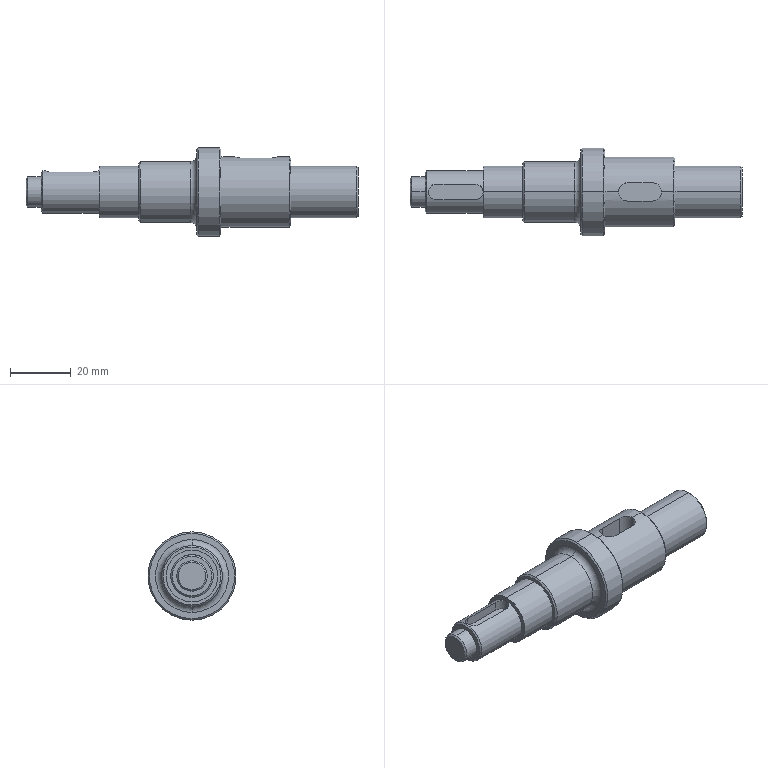Part | SolidWorks | features ICE 8, Chamfer 1, Extrusion 1, Fillet 1 | 1 solid | 50 faces | box 109 x 29 x 29 mm | volume 31302 mm3 | cylinder 20 | cone 14 | plane 14 | torus 2 | commonest cylinder face diameters 17 x4 5 x3 6 x3 10 x2 14 x2 20 x2
STEP:
#1=CARTESIAN_POINT('',(56.,0.,12.));
#2=VERTEX_POINT('',#1);
#3=CARTESIAN_POINT('',(56.,0.,-12.));
#4=VERTEX_POINT('',#3);
#5=CARTESIAN_POINT('',(56.,0.,0.));
#6=DIRECTION('',(1.,0.,0.));
#7=DIRECTION('',(0.,0.,-1.));
#8=AXIS2_PLACEMENT_3D('',#5,#6,#7);
#9=CIRCLE('',#8,12.);
#10=EDGE_CURVE('',#2,#4,#9,.T.);
#11=ORIENTED_EDGE('',*,*,#10,.F.);
#12=CARTESIAN_POINT('',(54.,0.,10.));
#13=VERTEX_POINT('',#12);
#14=CARTESIAN_POINT('',(54.,0.,12.));
#15=DIRECTION('',(0.,1.,0.));
#16=DIRECTION('',(0.,0.,1.));
#17=AXIS2_PLACEMENT_3D('',#14,#15,#16);
#18=CIRCLE('',#17,2.);
#19=EDGE_CURVE('',#2,#13,#18,.T.);
#20=ORIENTED_EDGE('',*,*,#19,.T.);
#21=CARTESIAN_POINT('',(54.,0.,-10.));
#22=VERTEX_POINT('',#21);
#23=CARTESIAN_POINT('',(54.,0.,0.));
#24=DIRECTION('',(-1.,0.,0.));
#25=DIRECTION('',(0.,0.,-1.));
#26=AXIS2_PLACEMENT_3D('',#23,#24,#25);
#27=CIRCLE('',#26,10.);
#28=EDGE_CURVE('',#22,#13,#27,.T.);
#29=ORIENTED_EDGE('',*,*,#28,.F.);
#30=CARTESIAN_POINT('',(54.,0.,-12.));
#31=DIRECTION('',(0.,-1.,0.));
#32=DIRECTION('',(0.,0.,-1.));
#33=AXIS2_PLACEMENT_3D('',#30,#31,#32);
#34=CIRCLE('',#33,2.);
#35=EDGE_CURVE('',#4,#22,#34,.T.);
#36=ORIENTED_EDGE('',*,*,#35,.F.);
#37=EDGE_LOOP('',(#11,#20,#29,#36));
#38=FACE_OUTER_BOUND('',#37,.T.);
#39=CARTESIAN_POINT('',(54.,0.,0.));
#40=DIRECTION('',(1.,0.,0.));
#41=DIRECTION('',(0.,0.,-1.));
#42=AXIS2_PLACEMENT_3D('',#39,#40,#41);
#43=TOROIDAL_SURFACE('',#42,12.,2.);
#44=ADVANCED_FACE('',(#38),#43,.F.);
#45=CARTESIAN_POINT('',(82.5,0.,5.));
#46=VERTEX_POINT('',#45);
#47=CARTESIAN_POINT('',(79.5,3.,5.));
#48=VERTEX_POINT('',#47);
#49=CARTESIAN_POINT('',(79.5,0.,5.));
#50=DIRECTION('',(0.,0.,1.));
#51=DIRECTION('',(1.,0.,0.));
#52=AXIS2_PLACEMENT_3D('',#49,#50,#51);
#53=CIRCLE('',#52,3.);
#54=EDGE_CURVE('',#46,#48,#53,.T.);
#55=ORIENTED_EDGE('',*,*,#54,.F.);
#56=CARTESIAN_POINT('',(82.5,0.,11.5));
#57=VERTEX_POINT('',#56);
#58=CARTESIAN_POINT('',(82.5,0.,5.));
#59=DIRECTION('',(0.,0.,1.));
#60=VECTOR('',#59,1000.);
#61=LINE('',#58,#60);
#62=EDGE_CURVE('',#46,#57,#61,.T.);
#63=ORIENTED_EDGE('',*,*,#62,.T.);
#64=CARTESIAN_POINT('',(79.5,3.,11.102));
#65=VERTEX_POINT('',#64);
#66=CARTESIAN_POINT('',(79.5,3.,11.102));
#67=CARTESIAN_POINT('',(79.699,3.,11.102));
#68=CARTESIAN_POINT('',(79.895,2.98,11.107));
#69=CARTESIAN_POINT('',(80.28,2.904,11.127));
#70=CARTESIAN_POINT('',(80.471,2.845,11.143));
#71=CARTESIAN_POINT('',(80.834,2.694,11.18));
#72=CARTESIAN_POINT('',(81.006,2.602,11.202));
#73=CARTESIAN_POINT('',(81.331,2.384,11.251));
#74=CARTESIAN_POINT('',(81.485,2.258,11.277));
#75=CARTESIAN_POINT('',(81.76,1.983,11.329));
#76=CARTESIAN_POINT('',(81.884,1.832,11.354));
#77=CARTESIAN_POINT('',(82.103,1.504,11.402));
#78=CARTESIAN_POINT('',(82.196,1.331,11.424));
#79=CARTESIAN_POINT('',(82.346,0.97,11.46));
#80=CARTESIAN_POINT('',(82.404,0.7798,11.475));
#81=CARTESIAN_POINT('',(82.481,0.392,11.495));
#82=CARTESIAN_POINT('',(82.5,0.1967,11.5));
#83=CARTESIAN_POINT('',(82.5,0.,11.5));
#84=B_SPLINE_CURVE_WITH_KNOTS('',3,(#66,#67,#68,#69,#70,#71,#72,#73,#74,#75,#76,#77,#78,#79,#80,#81,#82,#83),.UNSPECIFIED.,.F.,.F.,(4,2,2,2,2,2,2,2,4),(0.,0.0005889,0.001178,0.001767,0.002356,0.002945,0.003533,0.004122,0.004711),.UNSPECIFIED.);
#85=EDGE_CURVE('',#65,#57,#84,.T.);
#86=ORIENTED_EDGE('',*,*,#85,.F.);
#87=CARTESIAN_POINT('',(79.5,3.,5.));
#88=DIRECTION('',(0.,0.,1.));
#89=VECTOR('',#88,1000.);
#90=LINE('',#87,#89);
#91=EDGE_CURVE('',#48,#65,#90,.T.);
#92=ORIENTED_EDGE('',*,*,#91,.F.);
#93=EDGE_LOOP('',(#55,#63,#86,#92));
#94=FACE_OUTER_BOUND('',#93,.T.);
#95=CARTESIAN_POINT('',(79.5,0.,5.));
#96=DIRECTION('',(0.,0.,1.));
#97=DIRECTION('',(1.,0.,0.));
#98=AXIS2_PLACEMENT_3D('',#95,#96,#97);
#99=CYLINDRICAL_SURFACE('',#98,3.);
#100=ADVANCED_FACE('',(#94),#99,.F.);
#101=CARTESIAN_POINT('',(24.,0.,3.5));
#102=VERTEX_POINT('',#101);
#103=CARTESIAN_POINT('',(21.5,2.5,3.5));
#104=VERTEX_POINT('',#103);
#105=CARTESIAN_POINT('',(21.5,0.,3.5));
#106=DIRECTION('',(0.,0.,1.));
#107=DIRECTION('',(1.,0.,0.));
#108=AXIS2_PLACEMENT_3D('',#105,#106,#107);
#109=CIRCLE('',#108,2.5);
#110=EDGE_CURVE('',#102,#104,#109,.T.);
#111=ORIENTED_EDGE('',*,*,#110,.F.);
#112=CARTESIAN_POINT('',(24.,0.,7.));
#113=VERTEX_POINT('',#112);
#114=CARTESIAN_POINT('',(24.,0.,3.5));
#115=DIRECTION('',(0.,0.,1.));
#116=VECTOR('',#115,1000.);
#117=LINE('',#114,#116);
#118=EDGE_CURVE('',#102,#113,#117,.T.);
#119=ORIENTED_EDGE('',*,*,#118,.T.);
#120=CARTESIAN_POINT('',(21.5,2.5,6.538));
#121=VERTEX_POINT('',#120);
#122=CARTESIAN_POINT('',(21.5,2.5,6.538));
#123=CARTESIAN_POINT('',(21.667,2.5,6.538));
#124=CARTESIAN_POINT('',(21.83,2.484,6.545));
#125=CARTESIAN_POINT('',(22.151,2.419,6.569));
#126=CARTESIAN_POINT('',(22.311,2.371,6.587));
#127=CARTESIAN_POINT('',(22.612,2.245,6.631));
#128=CARTESIAN_POINT('',(22.755,2.168,6.656));
#129=CARTESIAN_POINT('',(23.026,1.987,6.713));
#130=CARTESIAN_POINT('',(23.153,1.883,6.743));
#131=CARTESIAN_POINT('',(23.496,1.54,6.833));
#132=CARTESIAN_POINT('',(23.681,1.264,6.892));
#133=CARTESIAN_POINT('',(23.87,0.8135,6.954));
#134=CARTESIAN_POINT('',(23.918,0.6548,6.971));
#135=CARTESIAN_POINT('',(23.984,0.3308,6.994));
#136=CARTESIAN_POINT('',(24.,0.1666,7.));
#137=CARTESIAN_POINT('',(24.,0.,7.));
#138=B_SPLINE_CURVE_WITH_KNOTS('',3,(#122,#123,#124,#125,#126,#127,#128,#129,#130,#131,#132,#133,#134,#135,#136,#137),.UNSPECIFIED.,.F.,.F.,(4,2,2,2,2,2,2,4),(0.,0.0004923,0.0009846,0.001477,0.001969,0.002954,0.003446,0.003938),.UNSPECIFIED.);
#139=EDGE_CURVE('',#121,#113,#138,.T.);
#140=ORIENTED_EDGE('',*,*,#139,.F.);
#141=CARTESIAN_POINT('',(21.5,2.5,3.5));
#142=DIRECTION('',(0.,0.,1.));
#143=VECTOR('',#142,1000.);
#144=LINE('',#141,#143);
#145=EDGE_CURVE('',#104,#121,#144,.T.);
#146=ORIENTED_EDGE('',*,*,#145,.F.);
#147=EDGE_LOOP('',(#111,#119,#140,#146));
#148=FACE_OUTER_BOUND('',#147,.T.);
#149=CARTESIAN_POINT('',(21.5,0.,3.5));
#150=DIRECTION('',(0.,0.,1.));
#151=DIRECTION('',(1.,0.,0.));
#152=AXIS2_PLACEMENT_3D('',#149,#150,#151);
#153=CYLINDRICAL_SURFACE('',#152,2.5);
#154=ADVANCED_FACE('',(#148),#153,.F.);
#155=CARTESIAN_POINT('',(5.,0.,6.5));
#156=VERTEX_POINT('',#155);
#157=CARTESIAN_POINT('',(5.,0.,-6.5));
#158=VERTEX_POINT('',#157);
#159=CARTESIAN_POINT('',(5.,0.,0.));
#160=DIRECTION('',(-1.,0.,0.));
#161=DIRECTION('',(0.,0.,-1.));
#162=AXIS2_PLACEMENT_3D('',#159,#160,#161);
#163=CIRCLE('',#162,6.5);
#164=EDGE_CURVE('',#156,#158,#163,.T.);
#165=ORIENTED_EDGE('',*,*,#164,.F.);
#166=CARTESIAN_POINT('',(5.5,0.,7.));
#167=VERTEX_POINT('',#166);
#168=CARTESIAN_POINT('',(5.5,0.,7.));
#169=DIRECTION('',(0.7071,0.,0.7071));
#170=VECTOR('',#169,1000.);
#171=LINE('',#168,#170);
#172=EDGE_CURVE('',#156,#167,#171,.T.);
#173=ORIENTED_EDGE('',*,*,#172,.T.);
#174=CARTESIAN_POINT('',(5.5,0.,-7.));
#175=VERTEX_POINT('',#174);
#176=CARTESIAN_POINT('',(5.5,0.,0.));
#177=DIRECTION('',(1.,0.,0.));
#178=DIRECTION('',(0.,0.,-1.));
#179=AXIS2_PLACEMENT_3D('',#176,#177,#178);
#180=CIRCLE('',#179,7.);
#181=EDGE_CURVE('',#175,#167,#180,.T.);
#182=ORIENTED_EDGE('',*,*,#181,.F.);
#183=CARTESIAN_POINT('',(5.5,0.,-7.));
#184=DIRECTION('',(0.7071,0.,-0.7071));
#185=VECTOR('',#184,1000.);
#186=LINE('',#183,#185);
#187=EDGE_CURVE('',#158,#175,#186,.T.);
#188=ORIENTED_EDGE('',*,*,#187,.F.);
#189=EDGE_LOOP('',(#165,#173,#182,#188));
#190=FACE_OUTER_BOUND('',#189,.T.);
#191=CARTESIAN_POINT('',(5.5,0.,0.));
#192=DIRECTION('',(1.,0.,0.));
#193=DIRECTION('',(0.,0.,-1.));
#194=AXIS2_PLACEMENT_3D('',#191,#192,#193);
#195=CONICAL_SURFACE('',#194,7.,0.7854);
#196=ADVANCED_FACE('',(#190),#195,.T.);
#197=CARTESIAN_POINT('',(37.,0.,9.5));
#198=VERTEX_POINT('',#197);
#199=CARTESIAN_POINT('',(37.,0.,-9.5));
#200=VERTEX_POINT('',#199);
#201=CARTESIAN_POINT('',(37.,0.,0.));
#202=DIRECTION('',(-1.,0.,0.));
#203=DIRECTION('',(0.,0.,-1.));
#204=AXIS2_PLACEMENT_3D('',#201,#202,#203);
#205=CIRCLE('',#204,9.5);
#206=EDGE_CURVE('',#198,#200,#205,.T.);
#207=ORIENTED_EDGE('',*,*,#206,.F.);
#208=CARTESIAN_POINT('',(37.5,0.,10.));
#209=VERTEX_POINT('',#208);
#210=CARTESIAN_POINT('',(37.5,0.,10.));
#211=DIRECTION('',(0.7071,0.,0.7071));
#212=VECTOR('',#211,1000.);
#213=LINE('',#210,#212);
#214=EDGE_CURVE('',#198,#209,#213,.T.);
#215=ORIENTED_EDGE('',*,*,#214,.T.);
#216=CARTESIAN_POINT('',(37.5,0.,-10.));
#217=VERTEX_POINT('',#216);
#218=CARTESIAN_POINT('',(37.5,0.,0.));
#219=DIRECTION('',(1.,0.,0.));
#220=DIRECTION('',(0.,0.,-1.));
#221=AXIS2_PLACEMENT_3D('',#218,#219,#220);
#222=CIRCLE('',#221,10.);
#223=EDGE_CURVE('',#217,#209,#222,.T.);
#224=ORIENTED_EDGE('',*,*,#223,.F.);
#225=CARTESIAN_POINT('',(37.5,0.,-10.));
#226=DIRECTION('',(0.7071,0.,-0.7071));
#227=VECTOR('',#226,1000.);
#228=LINE('',#225,#227);
#229=EDGE_CURVE('',#200,#217,#228,.T.);
#230=ORIENTED_EDGE('',*,*,#229,.F.);
#231=EDGE_LOOP('',(#207,#215,#224,#230));
#232=FACE_OUTER_BOUND('',#231,.T.);
#233=CARTESIAN_POINT('',(37.5,0.,0.));
#234=DIRECTION('',(1.,0.,0.));
#235=DIRECTION('',(0.,0.,-1.));
#236=AXIS2_PLACEMENT_3D('',#233,#234,#235);
#237=CONICAL_SURFACE('',#236,10.,0.7854);
#238=ADVANCED_FACE('',(#232),#237,.T.);
#239=CARTESIAN_POINT('',(56.,0.,14.));
#240=VERTEX_POINT('',#239);
#241=CARTESIAN_POINT('',(56.,0.,-14.));
#242=VERTEX_POINT('',#241);
#243=CARTESIAN_POINT('',(56.,0.,0.));
#244=DIRECTION('',(-1.,0.,0.));
#245=DIRECTION('',(0.,0.,-1.));
#246=AXIS2_PLACEMENT_3D('',#243,#244,#245);
#247=CIRCLE('',#246,14.);
#248=EDGE_CURVE('',#240,#242,#247,.T.);
#249=ORIENTED_EDGE('',*,*,#248,.F.);
#250=CARTESIAN_POINT('',(56.5,0.,14.5));
#251=VERTEX_POINT('',#250);
#252=CARTESIAN_POINT('',(56.5,0.,14.5));
#253=DIRECTION('',(0.7071,0.,0.7071));
#254=VECTOR('',#253,1000.);
#255=LINE('',#252,#254);
#256=EDGE_CURVE('',#240,#251,#255,.T.);
#257=ORIENTED_EDGE('',*,*,#256,.T.);
#258=CARTESIAN_POINT('',(56.5,0.,-14.5));
#259=VERTEX_POINT('',#258);
#260=CARTESIAN_POINT('',(56.5,0.,0.));
#261=DIRECTION('',(1.,0.,0.));
#262=DIRECTION('',(0.,0.,-1.));
#263=AXIS2_PLACEMENT_3D('',#260,#261,#262);
#264=CIRCLE('',#263,14.5);
#265=EDGE_CURVE('',#259,#251,#264,.T.);
#266=ORIENTED_EDGE('',*,*,#265,.F.);
#267=CARTESIAN_POINT('',(56.5,0.,-14.5));
#268=DIRECTION('',(0.7071,0.,-0.7071));
#269=VECTOR('',#268,1000.);
#270=LINE('',#267,#269);
#271=EDGE_CURVE('',#242,#259,#270,.T.);
#272=ORIENTED_EDGE('',*,*,#271,.F.);
#273=EDGE_LOOP('',(#249,#257,#266,#272));
#274=FACE_OUTER_BOUND('',#273,.T.);
#275=CARTESIAN_POINT('',(56.5,0.,0.));
#276=DIRECTION('',(1.,0.,0.));
#277=DIRECTION('',(0.,0.,-1.));
#278=AXIS2_PLACEMENT_3D('',#275,#276,#277);
#279=CONICAL_SURFACE('',#278,14.5,0.7854);
#280=ADVANCED_FACE('',(#274),#279,.T.);
#281=CARTESIAN_POINT('',(64.,0.,-14.));
#282=VERTEX_POINT('',#281);
#283=CARTESIAN_POINT('',(64.,0.,14.));
#284=VERTEX_POINT('',#283);
#285=CARTESIAN_POINT('',(64.,0.,0.));
#286=DIRECTION('',(1.,0.,0.));
#287=DIRECTION('',(0.,0.,-1.));
#288=AXIS2_PLACEMENT_3D('',#285,#286,#287);
#289=CIRCLE('',#288,14.);
#290=EDGE_CURVE('',#282,#284,#289,.T.);
#291=ORIENTED_EDGE('',*,*,#290,.F.);
#292=CARTESIAN_POINT('',(63.5,0.,-14.5));
#293=VERTEX_POINT('',#292);
#294=CARTESIAN_POINT('',(64.,0.,-14.));
#295=DIRECTION('',(-0.7071,0.,-0.7071));
#296=VECTOR('',#295,1000.);
#297=LINE('',#294,#296);
#298=EDGE_CURVE('',#282,#293,#297,.T.);
#299=ORIENTED_EDGE('',*,*,#298,.T.);
#300=CARTESIAN_POINT('',(63.5,0.,14.5));
#301=VERTEX_POINT('',#300);
#302=CARTESIAN_POINT('',(63.5,0.,0.));
#303=DIRECTION('',(-1.,0.,0.));
#304=DIRECTION('',(0.,0.,-1.));
#305=AXIS2_PLACEMENT_3D('',#302,#303,#304);
#306=CIRCLE('',#305,14.5);
#307=EDGE_CURVE('',#301,#293,#306,.T.);
#308=ORIENTED_EDGE('',*,*,#307,.F.);
#309=CARTESIAN_POINT('',(64.,0.,14.));
#310=DIRECTION('',(-0.7071,0.,0.7071));
#311=VECTOR('',#310,1000.);
#312=LINE('',#309,#311);
#313=EDGE_CURVE('',#284,#301,#312,.T.);
#314=ORIENTED_EDGE('',*,*,#313,.F.);
#315=EDGE_LOOP('',(#291,#299,#308,#314));
#316=FACE_OUTER_BOUND('',#315,.T.);
#317=CARTESIAN_POINT('',(64.,0.,0.));
#318=DIRECTION('',(-1.,0.,0.));
#319=DIRECTION('',(0.,0.,1.));
#320=AXIS2_PLACEMENT_3D('',#317,#318,#319);
#321=CONICAL_SURFACE('',#320,14.,0.7854);
#322=ADVANCED_FACE('',(#316),#321,.T.);
#323=CARTESIAN_POINT('',(87.,0.,-11.));
#324=VERTEX_POINT('',#323);
#325=CARTESIAN_POINT('',(87.,0.,11.));
#326=VERTEX_POINT('',#325);
#327=CARTESIAN_POINT('',(87.,0.,0.));
#328=DIRECTION('',(1.,0.,0.));
#329=DIRECTION('',(0.,0.,-1.));
#330=AXIS2_PLACEMENT_3D('',#327,#328,#329);
#331=CIRCLE('',#330,11.);
#332=EDGE_CURVE('',#324,#326,#331,.T.);
#333=ORIENTED_EDGE('',*,*,#332,.F.);
#334=CARTESIAN_POINT('',(86.5,0.,-11.5));
#335=VERTEX_POINT('',#334);
#336=CARTESIAN_POINT('',(87.,0.,-11.));
#337=DIRECTION('',(-0.7071,0.,-0.7071));
#338=VECTOR('',#337,1000.);
#339=LINE('',#336,#338);
#340=EDGE_CURVE('',#324,#335,#339,.T.);
#341=ORIENTED_EDGE('',*,*,#340,.T.);
#342=CARTESIAN_POINT('',(86.5,0.,11.5));
#343=VERTEX_POINT('',#342);
#344=CARTESIAN_POINT('',(86.5,0.,0.));
#345=DIRECTION('',(-1.,0.,0.));
#346=DIRECTION('',(0.,0.,-1.));
#347=AXIS2_PLACEMENT_3D('',#344,#345,#346);
#348=CIRCLE('',#347,11.5);
#349=EDGE_CURVE('',#343,#335,#348,.T.);
#350=ORIENTED_EDGE('',*,*,#349,.F.);
#351=CARTESIAN_POINT('',(87.,0.,11.));
#352=DIRECTION('',(-0.7071,0.,0.7071));
#353=VECTOR('',#352,1000.);
#354=LINE('',#351,#353);
#355=EDGE_CURVE('',#326,#343,#354,.T.);
#356=ORIENTED_EDGE('',*,*,#355,.F.);
#357=EDGE_LOOP('',(#333,#341,#350,#356));
#358=FACE_OUTER_BOUND('',#357,.T.);
#359=CARTESIAN_POINT('',(87.,0.,0.));
#360=DIRECTION('',(-1.,0.,0.));
#361=DIRECTION('',(0.,0.,1.));
#362=AXIS2_PLACEMENT_3D('',#359,#360,#361);
#363=CONICAL_SURFACE('',#362,11.,0.7854);
#364=ADVANCED_FACE('',(#358),#363,.T.);
#365=CARTESIAN_POINT('',(109.,0.,-8.));
#366=VERTEX_POINT('',#365);
#367=CARTESIAN_POINT('',(109.,0.,8.));
#368=VERTEX_POINT('',#367);
#369=CARTESIAN_POINT('',(109.,0.,0.));
#370=DIRECTION('',(1.,0.,0.));
#371=DIRECTION('',(0.,0.,-1.));
#372=AXIS2_PLACEMENT_3D('',#369,#370,#371);
#373=CIRCLE('',#372,8.);
#374=EDGE_CURVE('',#366,#368,#373,.T.);
#375=ORIENTED_EDGE('',*,*,#374,.F.);
#376=CARTESIAN_POINT('',(108.5,0.,-8.5));
#377=VERTEX_POINT('',#376);
#378=CARTESIAN_POINT('',(109.,0.,-8.));
#379=DIRECTION('',(-0.7071,0.,-0.7071));
#380=VECTOR('',#379,1000.);
#381=LINE('',#378,#380);
#382=EDGE_CURVE('',#366,#377,#381,.T.);
#383=ORIENTED_EDGE('',*,*,#382,.T.);
#384=CARTESIAN_POINT('',(108.5,0.,8.5));
#385=VERTEX_POINT('',#384);
#386=CARTESIAN_POINT('',(108.5,0.,0.));
#387=DIRECTION('',(-1.,0.,0.));
#388=DIRECTION('',(0.,0.,-1.));
#389=AXIS2_PLACEMENT_3D('',#386,#387,#388);
#390=CIRCLE('',#389,8.5);
#391=EDGE_CURVE('',#385,#377,#390,.T.);
#392=ORIENTED_EDGE('',*,*,#391,.F.);
#393=CARTESIAN_POINT('',(109.,0.,8.));
#394=DIRECTION('',(-0.7071,0.,0.7071));
#395=VECTOR('',#394,1000.);
#396=LINE('',#393,#395);
#397=EDGE_CURVE('',#368,#385,#396,.T.);
#398=ORIENTED_EDGE('',*,*,#397,.F.);
#399=EDGE_LOOP('',(#375,#383,#392,#398));
#400=FACE_OUTER_BOUND('',#399,.T.);
#401=CARTESIAN_POINT('',(109.,0.,0.));
#402=DIRECTION('',(-1.,0.,0.));
#403=DIRECTION('',(0.,0.,1.));
#404=AXIS2_PLACEMENT_3D('',#401,#402,#403);
#405=CONICAL_SURFACE('',#404,8.,0.7854);
#406=ADVANCED_FACE('',(#400),#405,.T.);
#407=CARTESIAN_POINT('',(0.,0.,4.5));
#408=VERTEX_POINT('',#407);
#409=CARTESIAN_POINT('',(0.,0.,-4.5));
#410=VERTEX_POINT('',#409);
#411=CARTESIAN_POINT('',(0.,0.,0.));
#412=DIRECTION('',(-1.,0.,0.));
#413=DIRECTION('',(0.,0.,-1.));
#414=AXIS2_PLACEMENT_3D('',#411,#412,#413);
#415=CIRCLE('',#414,4.5);
#416=EDGE_CURVE('',#408,#410,#415,.T.);
#417=ORIENTED_EDGE('',*,*,#416,.F.);
#418=CARTESIAN_POINT('',(0.5,0.,5.));
#419=VERTEX_POINT('',#418);
#420=CARTESIAN_POINT('',(0.5,0.,5.));
#421=DIRECTION('',(0.7071,0.,0.7071));
#422=VECTOR('',#421,1000.);
#423=LINE('',#420,#422);
#424=EDGE_CURVE('',#408,#419,#423,.T.);
#425=ORIENTED_EDGE('',*,*,#424,.T.);
#426=CARTESIAN_POINT('',(0.5,0.,-5.));
#427=VERTEX_POINT('',#426);
#428=CARTESIAN_POINT('',(0.5,0.,0.));
#429=DIRECTION('',(1.,0.,0.));
#430=DIRECTION('',(0.,0.,-1.));
#431=AXIS2_PLACEMENT_3D('',#428,#429,#430);
#432=CIRCLE('',#431,5.);
#433=EDGE_CURVE('',#427,#419,#432,.T.);
#434=ORIENTED_EDGE('',*,*,#433,.F.);
#435=CARTESIAN_POINT('',(0.5,0.,-5.));
#436=DIRECTION('',(0.7071,0.,-0.7071));
#437=VECTOR('',#436,1000.);
#438=LINE('',#435,#437);
#439=EDGE_CURVE('',#410,#427,#438,.T.);
#440=ORIENTED_EDGE('',*,*,#439,.F.);
#441=EDGE_LOOP('',(#417,#425,#434,#440));
#442=FACE_OUTER_BOUND('',#441,.T.);
#443=CARTESIAN_POINT('',(0.5,0.,0.));
#444=DIRECTION('',(1.,0.,0.));
#445=DIRECTION('',(0.,0.,-1.));
#446=AXIS2_PLACEMENT_3D('',#443,#444,#445);
#447=CONICAL_SURFACE('',#446,5.,0.7854);
#448=ADVANCED_FACE('',(#442),#447,.T.);
#449=ORIENTED_EDGE('',*,*,#391,.T.);
#450=CARTESIAN_POINT('',(87.,0.,-8.5));
#451=VERTEX_POINT('',#450);
#452=CARTESIAN_POINT('',(109.,0.,-8.5));
#453=DIRECTION('',(-1.,0.,0.));
#454=VECTOR('',#453,1000.);
#455=LINE('',#452,#454);
#456=EDGE_CURVE('',#377,#451,#455,.T.);
#457=ORIENTED_EDGE('',*,*,#456,.T.);
#458=CARTESIAN_POINT('',(87.,0.,8.5));
#459=VERTEX_POINT('',#458);
#460=CARTESIAN_POINT('',(87.,0.,0.));
#461=DIRECTION('',(1.,0.,0.));
#462=DIRECTION('',(0.,0.,-1.));
#463=AXIS2_PLACEMENT_3D('',#460,#461,#462);
#464=CIRCLE('',#463,8.5);
#465=EDGE_CURVE('',#451,#459,#464,.T.);
#466=ORIENTED_EDGE('',*,*,#465,.T.);
#467=CARTESIAN_POINT('',(109.,0.,8.5));
#468=DIRECTION('',(-1.,0.,0.));
#469=VECTOR('',#468,1000.);
#470=LINE('',#467,#469);
#471=EDGE_CURVE('',#385,#459,#470,.T.);
#472=ORIENTED_EDGE('',*,*,#471,.F.);
#473=EDGE_LOOP('',(#449,#457,#466,#472));
#474=FACE_OUTER_BOUND('',#473,.T.);
#475=CARTESIAN_POINT('',(109.,0.,0.));
#476=DIRECTION('',(-1.,0.,0.));
#477=DIRECTION('',(0.,0.,1.));
#478=AXIS2_PLACEMENT_3D('',#475,#476,#477);
#479=CYLINDRICAL_SURFACE('',#478,8.5);
#480=ADVANCED_FACE('',(#474),#479,.T.);
#481=ORIENTED_EDGE('',*,*,#349,.T.);
#482=CARTESIAN_POINT('',(64.,0.,-11.5));
#483=VERTEX_POINT('',#482);
#484=CARTESIAN_POINT('',(87.,0.,-11.5));
#485=DIRECTION('',(-1.,0.,0.));
#486=VECTOR('',#485,1000.);
#487=LINE('',#484,#486);
#488=EDGE_CURVE('',#335,#483,#487,.T.);
#489=ORIENTED_EDGE('',*,*,#488,.T.);
#490=CARTESIAN_POINT('',(64.,0.,11.5));
#491=VERTEX_POINT('',#490);
#492=CARTESIAN_POINT('',(64.,0.,0.));
#493=DIRECTION('',(1.,0.,0.));
#494=DIRECTION('',(0.,0.,-1.));
#495=AXIS2_PLACEMENT_3D('',#492,#493,#494);
#496=CIRCLE('',#495,11.5);
#497=EDGE_CURVE('',#483,#491,#496,.T.);
#498=ORIENTED_EDGE('',*,*,#497,.T.);
#499=CARTESIAN_POINT('',(68.5,0.,11.5));
#500=VERTEX_POINT('',#499);
#501=CARTESIAN_POINT('',(87.,0.,11.5));
#502=DIRECTION('',(-1.,0.,0.));
#503=VECTOR('',#502,1000.);
#504=LINE('',#501,#503);
#505=EDGE_CURVE('',#500,#491,#504,.T.);
#506=ORIENTED_EDGE('',*,*,#505,.F.);
#507=CARTESIAN_POINT('',(71.5,3.,11.102));
#508=VERTEX_POINT('',#507);
#509=CARTESIAN_POINT('',(68.5,0.,11.5));
#510=CARTESIAN_POINT('',(68.5,0.1965,11.5));
#511=CARTESIAN_POINT('',(68.52,0.3961,11.495));
#512=CARTESIAN_POINT('',(68.597,0.7812,11.475));
#513=CARTESIAN_POINT('',(68.654,0.9685,11.461));
#514=CARTESIAN_POINT('',(68.881,1.515,11.406));
#515=CARTESIAN_POINT('',(69.101,1.844,11.355));
#516=CARTESIAN_POINT('',(69.518,2.26,11.277));
#517=CARTESIAN_POINT('',(69.668,2.384,11.251));
#518=CARTESIAN_POINT('',(69.992,2.601,11.203));
#519=CARTESIAN_POINT('',(70.167,2.695,11.18));
#520=CARTESIAN_POINT('',(70.529,2.845,11.143));
#521=CARTESIAN_POINT('',(70.716,2.902,11.128));
#522=CARTESIAN_POINT('',(71.102,2.98,11.107));
#523=CARTESIAN_POINT('',(71.301,3.,11.102));
#524=CARTESIAN_POINT('',(71.5,3.,11.102));
#525=B_SPLINE_CURVE_WITH_KNOTS('',3,(#509,#510,#511,#512,#513,#514,#515,#516,#517,#518,#519,#520,#521,#522,#523,#524),.UNSPECIFIED.,.F.,.F.,(4,2,2,2,2,2,2,4),(0.004711,0.0053,0.005888,0.007064,0.007653,0.008241,0.008829,0.009417),.UNSPECIFIED.);
#526=EDGE_CURVE('',#500,#508,#525,.T.);
#527=ORIENTED_EDGE('',*,*,#526,.T.);
#528=CARTESIAN_POINT('',(87.,3.,11.102));
#529=DIRECTION('',(1.,0.,0.));
#530=VECTOR('',#529,1000.);
#531=LINE('',#528,#530);
#532=EDGE_CURVE('',#508,#65,#531,.T.);
#533=ORIENTED_EDGE('',*,*,#532,.T.);
#534=ORIENTED_EDGE('',*,*,#85,.T.);
#535=CARTESIAN_POINT('',(87.,0.,11.5));
#536=DIRECTION('',(-1.,0.,0.));
#537=VECTOR('',#536,1000.);
#538=LINE('',#535,#537);
#539=EDGE_CURVE('',#343,#57,#538,.T.);
#540=ORIENTED_EDGE('',*,*,#539,.F.);
#541=EDGE_LOOP('',(#481,#489,#498,#506,#527,#533,#534,#540));
#542=FACE_OUTER_BOUND('',#541,.T.);
#543=CARTESIAN_POINT('',(87.,0.,0.));
#544=DIRECTION('',(-1.,0.,0.));
#545=DIRECTION('',(0.,0.,1.));
#546=AXIS2_PLACEMENT_3D('',#543,#544,#545);
#547=CYLINDRICAL_SURFACE('',#546,11.5);
#548=ADVANCED_FACE('',(#542),#547,.T.);
#549=ORIENTED_EDGE('',*,*,#307,.T.);
#550=CARTESIAN_POINT('',(64.,0.,-14.5));
#551=DIRECTION('',(-1.,0.,0.));
#552=VECTOR('',#551,1000.);
#553=LINE('',#550,#552);
#554=EDGE_CURVE('',#293,#259,#553,.T.);
#555=ORIENTED_EDGE('',*,*,#554,.T.);
#556=ORIENTED_EDGE('',*,*,#265,.T.);
#557=CARTESIAN_POINT('',(64.,0.,14.5));
#558=DIRECTION('',(-1.,0.,0.));
#559=VECTOR('',#558,1000.);
#560=LINE('',#557,#559);
#561=EDGE_CURVE('',#301,#251,#560,.T.);
#562=ORIENTED_EDGE('',*,*,#561,.F.);
#563=EDGE_LOOP('',(#549,#555,#556,#562));
#564=FACE_OUTER_BOUND('',#563,.T.);
#565=CARTESIAN_POINT('',(64.,0.,0.));
#566=DIRECTION('',(-1.,0.,0.));
#567=DIRECTION('',(0.,0.,1.));
#568=AXIS2_PLACEMENT_3D('',#565,#566,#567);
#569=CYLINDRICAL_SURFACE('',#568,14.5);
#570=ADVANCED_FACE('',(#564),#569,.T.);
#571=CARTESIAN_POINT('',(54.,0.,0.));
#572=DIRECTION('',(-1.,0.,0.));
#573=DIRECTION('',(0.,0.,-1.));
#574=AXIS2_PLACEMENT_3D('',#571,#572,#573);
#575=CIRCLE('',#574,10.);
#576=EDGE_CURVE('',#13,#22,#575,.T.);
#577=ORIENTED_EDGE('',*,*,#576,.T.);
#578=CARTESIAN_POINT('',(56.,0.,-10.));
#579=DIRECTION('',(-1.,0.,0.));
#580=VECTOR('',#579,1000.);
#581=LINE('',#578,#580);
#582=EDGE_CURVE('',#22,#217,#581,.T.);
#583=ORIENTED_EDGE('',*,*,#582,.T.);
#584=ORIENTED_EDGE('',*,*,#223,.T.);
#585=CARTESIAN_POINT('',(56.,0.,10.));
#586=DIRECTION('',(-1.,0.,0.));
#587=VECTOR('',#586,1000.);
#588=LINE('',#585,#587);
#589=EDGE_CURVE('',#13,#209,#588,.T.);
#590=ORIENTED_EDGE('',*,*,#589,.F.);
#591=EDGE_LOOP('',(#577,#583,#584,#590));
#592=FACE_OUTER_BOUND('',#591,.T.);
#593=CARTESIAN_POINT('',(56.,0.,0.));
#594=DIRECTION('',(-1.,0.,0.));
#595=DIRECTION('',(0.,0.,1.));
#596=AXIS2_PLACEMENT_3D('',#593,#594,#595);
#597=CYLINDRICAL_SURFACE('',#596,10.);
#598=ADVANCED_FACE('',(#592),#597,.T.);
#599=CARTESIAN_POINT('',(37.,0.,-8.5));
#600=VERTEX_POINT('',#599);
#601=CARTESIAN_POINT('',(37.,0.,8.5));
#602=VERTEX_POINT('',#601);
#603=CARTESIAN_POINT('',(37.,0.,0.));
#604=DIRECTION('',(1.,0.,0.));
#605=DIRECTION('',(0.,0.,-1.));
#606=AXIS2_PLACEMENT_3D('',#603,#604,#605);
#607=CIRCLE('',#606,8.5);
#608=EDGE_CURVE('',#600,#602,#607,.T.);
#609=ORIENTED_EDGE('',*,*,#608,.F.);
#610=CARTESIAN_POINT('',(24.,0.,-8.5));
#611=VERTEX_POINT('',#610);
#612=CARTESIAN_POINT('',(37.,0.,-8.5));
#613=DIRECTION('',(-1.,0.,0.));
#614=VECTOR('',#613,1000.);
#615=LINE('',#612,#614);
#616=EDGE_CURVE('',#600,#611,#615,.T.);
#617=ORIENTED_EDGE('',*,*,#616,.T.);
#618=CARTESIAN_POINT('',(24.,0.,8.5));
#619=VERTEX_POINT('',#618);
#620=CARTESIAN_POINT('',(24.,0.,0.));
#621=DIRECTION('',(1.,0.,0.));
#622=DIRECTION('',(0.,0.,-1.));
#623=AXIS2_PLACEMENT_3D('',#620,#621,#622);
#624=CIRCLE('',#623,8.5);
#625=EDGE_CURVE('',#611,#619,#624,.T.);
#626=ORIENTED_EDGE('',*,*,#625,.T.);
#627=CARTESIAN_POINT('',(37.,0.,8.5));
#628=DIRECTION('',(-1.,0.,0.));
#629=VECTOR('',#628,1000.);
#630=LINE('',#627,#629);
#631=EDGE_CURVE('',#602,#619,#630,.T.);
#632=ORIENTED_EDGE('',*,*,#631,.F.);
#633=EDGE_LOOP('',(#609,#617,#626,#632));
#634=FACE_OUTER_BOUND('',#633,.T.);
#635=CARTESIAN_POINT('',(37.,0.,0.));
#636=DIRECTION('',(-1.,0.,0.));
#637=DIRECTION('',(0.,0.,1.));
#638=AXIS2_PLACEMENT_3D('',#635,#636,#637);
#639=CYLINDRICAL_SURFACE('',#638,8.5);
#640=ADVANCED_FACE('',(#634),#639,.T.);
#641=CARTESIAN_POINT('',(24.,0.,-7.));
#642=VERTEX_POINT('',#641);
#643=CARTESIAN_POINT('',(24.,0.,0.));
#644=DIRECTION('',(1.,0.,0.));
#645=DIRECTION('',(0.,0.,-1.));
#646=AXIS2_PLACEMENT_3D('',#643,#644,#645);
#647=CIRCLE('',#646,7.);
#648=EDGE_CURVE('',#642,#113,#647,.T.);
#649=ORIENTED_EDGE('',*,*,#648,.F.);
#650=CARTESIAN_POINT('',(24.,0.,-7.));
#651=DIRECTION('',(-1.,0.,0.));
#652=VECTOR('',#651,1000.);
#653=LINE('',#650,#652);
#654=EDGE_CURVE('',#642,#175,#653,.T.);
#655=ORIENTED_EDGE('',*,*,#654,.T.);
#656=ORIENTED_EDGE('',*,*,#181,.T.);
#657=CARTESIAN_POINT('',(6.,0.,7.));
#658=VERTEX_POINT('',#657);
#659=CARTESIAN_POINT('',(24.,0.,7.));
#660=DIRECTION('',(-1.,0.,0.));
#661=VECTOR('',#660,1000.);
#662=LINE('',#659,#661);
#663=EDGE_CURVE('',#658,#167,#662,.T.);
#664=ORIENTED_EDGE('',*,*,#663,.F.);
#665=CARTESIAN_POINT('',(8.5,2.5,6.538));
#666=VERTEX_POINT('',#665);
#667=CARTESIAN_POINT('',(6.,0.,7.));
#668=CARTESIAN_POINT('',(6.,0.1645,7.));
#669=CARTESIAN_POINT('',(6.017,0.3315,6.994));
#670=CARTESIAN_POINT('',(6.081,0.653,6.971));
#671=CARTESIAN_POINT('',(6.129,0.8095,6.955));
#672=CARTESIAN_POINT('',(6.256,1.114,6.913));
#673=CARTESIAN_POINT('',(6.333,1.257,6.888));
#674=CARTESIAN_POINT('',(6.514,1.527,6.833));
#675=CARTESIAN_POINT('',(6.618,1.654,6.803));
#676=CARTESIAN_POINT('',(6.848,1.883,6.743));
#677=CARTESIAN_POINT('',(6.972,1.986,6.713));
#678=CARTESIAN_POINT('',(7.242,2.166,6.657));
#679=CARTESIAN_POINT('',(7.388,2.245,6.631));
#680=CARTESIAN_POINT('',(7.688,2.37,6.587));
#681=CARTESIAN_POINT('',(7.844,2.418,6.569));
#682=CARTESIAN_POINT('',(8.167,2.483,6.545));
#683=CARTESIAN_POINT('',(8.333,2.5,6.538));
#684=CARTESIAN_POINT('',(8.5,2.5,6.538));
#685=B_SPLINE_CURVE_WITH_KNOTS('',3,(#667,#668,#669,#670,#671,#672,#673,#674,#675,#676,#677,#678,#679,#680,#681,#682,#683,#684),.UNSPECIFIED.,.F.,.F.,(4,2,2,2,2,2,2,2,4),(0.003942,0.004434,0.004926,0.005418,0.00591,0.006402,0.006894,0.007386,0.007878),.UNSPECIFIED.);
#686=EDGE_CURVE('',#658,#666,#685,.T.);
#687=ORIENTED_EDGE('',*,*,#686,.T.);
#688=CARTESIAN_POINT('',(24.,2.5,6.538));
#689=DIRECTION('',(1.,0.,0.));
#690=VECTOR('',#689,1000.);
#691=LINE('',#688,#690);
#692=EDGE_CURVE('',#666,#121,#691,.T.);
#693=ORIENTED_EDGE('',*,*,#692,.T.);
#694=ORIENTED_EDGE('',*,*,#139,.T.);
#695=EDGE_LOOP('',(#649,#655,#656,#664,#687,#693,#694));
#696=FACE_OUTER_BOUND('',#695,.T.);
#697=CARTESIAN_POINT('',(24.,0.,0.));
#698=DIRECTION('',(-1.,0.,0.));
#699=DIRECTION('',(0.,0.,1.));
#700=AXIS2_PLACEMENT_3D('',#697,#698,#699);
#701=CYLINDRICAL_SURFACE('',#700,7.);
#702=ADVANCED_FACE('',(#696),#701,.T.);
#703=CARTESIAN_POINT('',(5.,0.,-5.));
#704=VERTEX_POINT('',#703);
#705=CARTESIAN_POINT('',(5.,0.,5.));
#706=VERTEX_POINT('',#705);
#707=CARTESIAN_POINT('',(5.,0.,0.));
#708=DIRECTION('',(1.,0.,0.));
#709=DIRECTION('',(0.,0.,-1.));
#710=AXIS2_PLACEMENT_3D('',#707,#708,#709);
#711=CIRCLE('',#710,5.);
#712=EDGE_CURVE('',#704,#706,#711,.T.);
#713=ORIENTED_EDGE('',*,*,#712,.F.);
#714=CARTESIAN_POINT('',(5.,0.,-5.));
#715=DIRECTION('',(-1.,0.,0.));
#716=VECTOR('',#715,1000.);
#717=LINE('',#714,#716);
#718=EDGE_CURVE('',#704,#427,#717,.T.);
#719=ORIENTED_EDGE('',*,*,#718,.T.);
#720=ORIENTED_EDGE('',*,*,#433,.T.);
#721=CARTESIAN_POINT('',(5.,0.,5.));
#722=DIRECTION('',(-1.,0.,0.));
#723=VECTOR('',#722,1000.);
#724=LINE('',#721,#723);
#725=EDGE_CURVE('',#706,#419,#724,.T.);
#726=ORIENTED_EDGE('',*,*,#725,.F.);
#727=EDGE_LOOP('',(#713,#719,#720,#726));
#728=FACE_OUTER_BOUND('',#727,.T.);
#729=CARTESIAN_POINT('',(5.,0.,0.));
#730=DIRECTION('',(-1.,0.,0.));
#731=DIRECTION('',(0.,0.,1.));
#732=AXIS2_PLACEMENT_3D('',#729,#730,#731);
#733=CYLINDRICAL_SURFACE('',#732,5.);
#734=ADVANCED_FACE('',(#728),#733,.T.);
#735=ORIENTED_EDGE('',*,*,#718,.F.);
#736=CARTESIAN_POINT('',(5.,0.,0.));
#737=DIRECTION('',(1.,0.,0.));
#738=DIRECTION('',(0.,0.,-1.));
#739=AXIS2_PLACEMENT_3D('',#736,#737,#738);
#740=CIRCLE('',#739,5.);
#741=EDGE_CURVE('',#706,#704,#740,.T.);
#742=ORIENTED_EDGE('',*,*,#741,.F.);
#743=ORIENTED_EDGE('',*,*,#725,.T.);
#744=CARTESIAN_POINT('',(0.5,0.,0.));
#745=DIRECTION('',(1.,0.,0.));
#746=DIRECTION('',(0.,0.,-1.));
#747=AXIS2_PLACEMENT_3D('',#744,#745,#746);
#748=CIRCLE('',#747,5.);
#749=EDGE_CURVE('',#419,#427,#748,.T.);
#750=ORIENTED_EDGE('',*,*,#749,.T.);
#751=EDGE_LOOP('',(#735,#742,#743,#750));
#752=FACE_OUTER_BOUND('',#751,.T.);
#753=CARTESIAN_POINT('',(5.,0.,0.));
#754=DIRECTION('',(-1.,0.,0.));
#755=DIRECTION('',(0.,0.,1.));
#756=AXIS2_PLACEMENT_3D('',#753,#754,#755);
#757=CYLINDRICAL_SURFACE('',#756,5.);
#758=ADVANCED_FACE('',(#752),#757,.T.);
#759=CARTESIAN_POINT('',(0.,0.,0.));
#760=DIRECTION('',(-1.,0.,0.));
#761=DIRECTION('',(0.,0.,-1.));
#762=AXIS2_PLACEMENT_3D('',#759,#760,#761);
#763=CIRCLE('',#762,4.5);
#764=EDGE_CURVE('',#410,#408,#763,.T.);
#765=ORIENTED_EDGE('',*,*,#764,.T.);
#766=ORIENTED_EDGE('',*,*,#416,.T.);
#767=EDGE_LOOP('',(#765,#766));
#768=FACE_OUTER_BOUND('',#767,.T.);
#769=CARTESIAN_POINT('',(0.,0.,0.));
#770=DIRECTION('',(1.,0.,0.));
#771=DIRECTION('',(0.,0.,-1.));
#772=AXIS2_PLACEMENT_3D('',#769,#770,#771);
#773=PLANE('',#772);
#774=ADVANCED_FACE('',(#768),#773,.F.);
#775=ORIENTED_EDGE('',*,*,#654,.F.);
#776=CARTESIAN_POINT('',(24.,0.,0.));
#777=DIRECTION('',(1.,0.,0.));
#778=DIRECTION('',(0.,0.,-1.));
#779=AXIS2_PLACEMENT_3D('',#776,#777,#778);
#780=CIRCLE('',#779,7.);
#781=EDGE_CURVE('',#113,#642,#780,.T.);
#782=ORIENTED_EDGE('',*,*,#781,.F.);
#783=CARTESIAN_POINT('',(21.5,-2.5,6.538));
#784=VERTEX_POINT('',#783);
#785=CARTESIAN_POINT('',(24.,0.,7.));
#786=CARTESIAN_POINT('',(24.,-0.1666,7.));
#787=CARTESIAN_POINT('',(23.984,-0.3301,6.994));
#788=CARTESIAN_POINT('',(23.919,-0.6514,6.971));
#789=CARTESIAN_POINT('',(23.871,-0.8108,6.955));
#790=CARTESIAN_POINT('',(23.745,-1.113,6.913));
#791=CARTESIAN_POINT('',(23.668,-1.256,6.888));
#792=CARTESIAN_POINT('',(23.486,-1.527,6.833));
#793=CARTESIAN_POINT('',(23.382,-1.654,6.803));
#794=CARTESIAN_POINT('',(23.039,-1.996,6.713));
#795=CARTESIAN_POINT('',(22.763,-2.182,6.653));
#796=CARTESIAN_POINT('',(22.313,-2.37,6.587));
#797=CARTESIAN_POINT('',(22.155,-2.418,6.569));
#798=CARTESIAN_POINT('',(21.831,-2.484,6.545));
#799=CARTESIAN_POINT('',(21.667,-2.5,6.538));
#800=CARTESIAN_POINT('',(21.5,-2.5,6.538));
#801=B_SPLINE_CURVE_WITH_KNOTS('',3,(#785,#786,#787,#788,#789,#790,#791,#792,#793,#794,#795,#796,#797,#798,#799,#800),.UNSPECIFIED.,.F.,.F.,(4,2,2,2,2,2,2,4),(0.,0.0004923,0.0009846,0.001477,0.001969,0.002954,0.003446,0.003938),.UNSPECIFIED.);
#802=EDGE_CURVE('',#113,#784,#801,.T.);
#803=ORIENTED_EDGE('',*,*,#802,.T.);
#804=CARTESIAN_POINT('',(8.5,-2.5,6.538));
#805=VERTEX_POINT('',#804);
#806=CARTESIAN_POINT('',(24.,-2.5,6.538));
#807=DIRECTION('',(-1.,0.,0.));
#808=VECTOR('',#807,1000.);
#809=LINE('',#806,#808);
#810=EDGE_CURVE('',#784,#805,#809,.T.);
#811=ORIENTED_EDGE('',*,*,#810,.T.);
#812=CARTESIAN_POINT('',(8.5,-2.5,6.538));
#813=CARTESIAN_POINT('',(8.333,-2.5,6.538));
#814=CARTESIAN_POINT('',(8.17,-2.483,6.545));
#815=CARTESIAN_POINT('',(7.848,-2.419,6.569));
#816=CARTESIAN_POINT('',(7.689,-2.37,6.587));
#817=CARTESIAN_POINT('',(7.387,-2.244,6.631));
#818=CARTESIAN_POINT('',(7.244,-2.167,6.657));
#819=CARTESIAN_POINT('',(6.973,-1.986,6.713));
#820=CARTESIAN_POINT('',(6.846,-1.881,6.743));
#821=CARTESIAN_POINT('',(6.503,-1.538,6.833));
#822=CARTESIAN_POINT('',(6.317,-1.262,6.892));
#823=CARTESIAN_POINT('',(6.129,-0.8107,6.955));
#824=CARTESIAN_POINT('',(6.081,-0.6515,6.971));
#825=CARTESIAN_POINT('',(6.016,-0.328,6.994));
#826=CARTESIAN_POINT('',(6.,-0.1647,7.));
#827=CARTESIAN_POINT('',(6.,0.,7.));
#828=B_SPLINE_CURVE_WITH_KNOTS('',3,(#812,#813,#814,#815,#816,#817,#818,#819,#820,#821,#822,#823,#824,#825,#826,#827),.UNSPECIFIED.,.F.,.F.,(4,2,2,2,2,2,2,4),(0.,0.0004927,0.0009855,0.001478,0.001971,0.002956,0.003449,0.003942),.UNSPECIFIED.);
#829=EDGE_CURVE('',#805,#658,#828,.T.);
#830=ORIENTED_EDGE('',*,*,#829,.T.);
#831=ORIENTED_EDGE('',*,*,#663,.T.);
#832=CARTESIAN_POINT('',(5.5,0.,0.));
#833=DIRECTION('',(1.,0.,0.));
#834=DIRECTION('',(0.,0.,-1.));
#835=AXIS2_PLACEMENT_3D('',#832,#833,#834);
#836=CIRCLE('',#835,7.);
#837=EDGE_CURVE('',#167,#175,#836,.T.);
#838=ORIENTED_EDGE('',*,*,#837,.T.);
#839=EDGE_LOOP('',(#775,#782,#803,#811,#830,#831,#838));
#840=FACE_OUTER_BOUND('',#839,.T.);
#841=CARTESIAN_POINT('',(24.,0.,0.));
#842=DIRECTION('',(-1.,0.,0.));
#843=DIRECTION('',(0.,0.,1.));
#844=AXIS2_PLACEMENT_3D('',#841,#842,#843);
#845=CYLINDRICAL_SURFACE('',#844,7.);
#846=ADVANCED_FACE('',(#840),#845,.T.);
#847=CARTESIAN_POINT('',(5.,0.,0.));
#848=DIRECTION('',(-1.,0.,0.));
#849=DIRECTION('',(0.,0.,-1.));
#850=AXIS2_PLACEMENT_3D('',#847,#848,#849);
#851=CIRCLE('',#850,6.5);
#852=EDGE_CURVE('',#158,#156,#851,.T.);
#853=ORIENTED_EDGE('',*,*,#852,.T.);
#854=ORIENTED_EDGE('',*,*,#164,.T.);
#855=EDGE_LOOP('',(#853,#854));
#856=FACE_OUTER_BOUND('',#855,.T.);
#857=ORIENTED_EDGE('',*,*,#741,.T.);
#858=ORIENTED_EDGE('',*,*,#712,.T.);
#859=EDGE_LOOP('',(#857,#858));
#860=FACE_BOUND('',#859,.T.);
#861=CARTESIAN_POINT('',(5.,0.,0.));
#862=DIRECTION('',(1.,0.,0.));
#863=DIRECTION('',(0.,0.,-1.));
#864=AXIS2_PLACEMENT_3D('',#861,#862,#863);
#865=PLANE('',#864);
#866=ADVANCED_FACE('',(#856,#860),#865,.F.);
#867=ORIENTED_EDGE('',*,*,#616,.F.);
#868=CARTESIAN_POINT('',(37.,0.,0.));
#869=DIRECTION('',(1.,0.,0.));
#870=DIRECTION('',(0.,0.,-1.));
#871=AXIS2_PLACEMENT_3D('',#868,#869,#870);
#872=CIRCLE('',#871,8.5);
#873=EDGE_CURVE('',#602,#600,#872,.T.);
#874=ORIENTED_EDGE('',*,*,#873,.F.);
#875=ORIENTED_EDGE('',*,*,#631,.T.);
#876=CARTESIAN_POINT('',(24.,0.,0.));
#877=DIRECTION('',(1.,0.,0.));
#878=DIRECTION('',(0.,0.,-1.));
#879=AXIS2_PLACEMENT_3D('',#876,#877,#878);
#880=CIRCLE('',#879,8.5);
#881=EDGE_CURVE('',#619,#611,#880,.T.);
#882=ORIENTED_EDGE('',*,*,#881,.T.);
#883=EDGE_LOOP('',(#867,#874,#875,#882));
#884=FACE_OUTER_BOUND('',#883,.T.);
#885=CARTESIAN_POINT('',(37.,0.,0.));
#886=DIRECTION('',(-1.,0.,0.));
#887=DIRECTION('',(0.,0.,1.));
#888=AXIS2_PLACEMENT_3D('',#885,#886,#887);
#889=CYLINDRICAL_SURFACE('',#888,8.5);
#890=ADVANCED_FACE('',(#884),#889,.T.);
#891=ORIENTED_EDGE('',*,*,#781,.T.);
#892=ORIENTED_EDGE('',*,*,#648,.T.);
#893=EDGE_LOOP('',(#891,#892));
#894=FACE_BOUND('',#893,.T.);
#895=ORIENTED_EDGE('',*,*,#881,.F.);
#896=ORIENTED_EDGE('',*,*,#625,.F.);
#897=EDGE_LOOP('',(#895,#896));
#898=FACE_OUTER_BOUND('',#897,.T.);
#899=CARTESIAN_POINT('',(24.,0.,0.));
#900=DIRECTION('',(1.,0.,0.));
#901=DIRECTION('',(0.,0.,-1.));
#902=AXIS2_PLACEMENT_3D('',#899,#900,#901);
#903=PLANE('',#902);
#904=ADVANCED_FACE('',(#894,#898),#903,.F.);
#905=ORIENTED_EDGE('',*,*,#582,.F.);
#906=ORIENTED_EDGE('',*,*,#28,.T.);
#907=ORIENTED_EDGE('',*,*,#589,.T.);
#908=CARTESIAN_POINT('',(37.5,0.,0.));
#909=DIRECTION('',(1.,0.,0.));
#910=DIRECTION('',(0.,0.,-1.));
#911=AXIS2_PLACEMENT_3D('',#908,#909,#910);
#912=CIRCLE('',#911,10.);
#913=EDGE_CURVE('',#209,#217,#912,.T.);
#914=ORIENTED_EDGE('',*,*,#913,.T.);
#915=EDGE_LOOP('',(#905,#906,#907,#914));
#916=FACE_OUTER_BOUND('',#915,.T.);
#917=CARTESIAN_POINT('',(56.,0.,0.));
#918=DIRECTION('',(-1.,0.,0.));
#919=DIRECTION('',(0.,0.,1.));
#920=AXIS2_PLACEMENT_3D('',#917,#918,#919);
#921=CYLINDRICAL_SURFACE('',#920,10.);
#922=ADVANCED_FACE('',(#916),#921,.T.);
#923=CARTESIAN_POINT('',(37.,0.,0.));
#924=DIRECTION('',(-1.,0.,0.));
#925=DIRECTION('',(0.,0.,-1.));
#926=AXIS2_PLACEMENT_3D('',#923,#924,#925);
#927=CIRCLE('',#926,9.5);
#928=EDGE_CURVE('',#200,#198,#927,.T.);
#929=ORIENTED_EDGE('',*,*,#928,.T.);
#930=ORIENTED_EDGE('',*,*,#206,.T.);
#931=EDGE_LOOP('',(#929,#930));
#932=FACE_OUTER_BOUND('',#931,.T.);
#933=ORIENTED_EDGE('',*,*,#873,.T.);
#934=ORIENTED_EDGE('',*,*,#608,.T.);
#935=EDGE_LOOP('',(#933,#934));
#936=FACE_BOUND('',#935,.T.);
#937=CARTESIAN_POINT('',(37.,0.,0.));
#938=DIRECTION('',(1.,0.,0.));
#939=DIRECTION('',(0.,0.,-1.));
#940=AXIS2_PLACEMENT_3D('',#937,#938,#939);
#941=PLANE('',#940);
#942=ADVANCED_FACE('',(#932,#936),#941,.F.);
#943=ORIENTED_EDGE('',*,*,#554,.F.);
#944=CARTESIAN_POINT('',(63.5,0.,0.));
#945=DIRECTION('',(-1.,0.,0.));
#946=DIRECTION('',(0.,0.,-1.));
#947=AXIS2_PLACEMENT_3D('',#944,#945,#946);
#948=CIRCLE('',#947,14.5);
#949=EDGE_CURVE('',#293,#301,#948,.T.);
#950=ORIENTED_EDGE('',*,*,#949,.T.);
#951=ORIENTED_EDGE('',*,*,#561,.T.);
#952=CARTESIAN_POINT('',(56.5,0.,0.));
#953=DIRECTION('',(1.,0.,0.));
#954=DIRECTION('',(0.,0.,-1.));
#955=AXIS2_PLACEMENT_3D('',#952,#953,#954);
#956=CIRCLE('',#955,14.5);
#957=EDGE_CURVE('',#251,#259,#956,.T.);
#958=ORIENTED_EDGE('',*,*,#957,.T.);
#959=EDGE_LOOP('',(#943,#950,#951,#958));
#960=FACE_OUTER_BOUND('',#959,.T.);
#961=CARTESIAN_POINT('',(64.,0.,0.));
#962=DIRECTION('',(-1.,0.,0.));
#963=DIRECTION('',(0.,0.,1.));
#964=AXIS2_PLACEMENT_3D('',#961,#962,#963);
#965=CYLINDRICAL_SURFACE('',#964,14.5);
#966=ADVANCED_FACE('',(#960),#965,.T.);
#967=CARTESIAN_POINT('',(64.,0.,0.));
#968=DIRECTION('',(1.,0.,0.));
#969=DIRECTION('',(0.,0.,-1.));
#970=AXIS2_PLACEMENT_3D('',#967,#968,#969);
#971=CIRCLE('',#970,14.);
#972=EDGE_CURVE('',#284,#282,#971,.T.);
#973=ORIENTED_EDGE('',*,*,#972,.T.);
#974=ORIENTED_EDGE('',*,*,#290,.T.);
#975=EDGE_LOOP('',(#973,#974));
#976=FACE_OUTER_BOUND('',#975,.T.);
#977=CARTESIAN_POINT('',(64.,0.,0.));
#978=DIRECTION('',(1.,0.,0.));
#979=DIRECTION('',(0.,0.,-1.));
#980=AXIS2_PLACEMENT_3D('',#977,#978,#979);
#981=CIRCLE('',#980,11.5);
#982=EDGE_CURVE('',#491,#483,#981,.T.);
#983=ORIENTED_EDGE('',*,*,#982,.F.);
#984=ORIENTED_EDGE('',*,*,#497,.F.);
#985=EDGE_LOOP('',(#983,#984));
#986=FACE_BOUND('',#985,.T.);
#987=CARTESIAN_POINT('',(64.,0.,0.));
#988=DIRECTION('',(1.,0.,0.));
#989=DIRECTION('',(0.,0.,-1.));
#990=AXIS2_PLACEMENT_3D('',#987,#988,#989);
#991=PLANE('',#990);
#992=ADVANCED_FACE('',(#976,#986),#991,.T.);
#993=CARTESIAN_POINT('',(56.,0.,0.));
#994=DIRECTION('',(1.,0.,0.));
#995=DIRECTION('',(0.,0.,-1.));
#996=AXIS2_PLACEMENT_3D('',#993,#994,#995);
#997=CIRCLE('',#996,12.);
#998=EDGE_CURVE('',#4,#2,#997,.T.);
#999=ORIENTED_EDGE('',*,*,#998,.T.);
#1000=ORIENTED_EDGE('',*,*,#10,.T.);
#1001=EDGE_LOOP('',(#999,#1000));
#1002=FACE_BOUND('',#1001,.T.);
#1003=CARTESIAN_POINT('',(56.,0.,0.));
#1004=DIRECTION('',(-1.,0.,0.));
#1005=DIRECTION('',(0.,0.,-1.));
#1006=AXIS2_PLACEMENT_3D('',#1003,#1004,#1005);
#1007=CIRCLE('',#1006,14.);
#1008=EDGE_CURVE('',#242,#240,#1007,.T.);
#1009=ORIENTED_EDGE('',*,*,#1008,.T.);
#1010=ORIENTED_EDGE('',*,*,#248,.T.);
#1011=EDGE_LOOP('',(#1009,#1010));
#1012=FACE_OUTER_BOUND('',#1011,.T.);
#1013=CARTESIAN_POINT('',(56.,0.,0.));
#1014=DIRECTION('',(1.,0.,0.));
#1015=DIRECTION('',(0.,0.,-1.));
#1016=AXIS2_PLACEMENT_3D('',#1013,#1014,#1015);
#1017=PLANE('',#1016);
#1018=ADVANCED_FACE('',(#1002,#1012),#1017,.F.);
#1019=ORIENTED_EDGE('',*,*,#488,.F.);
#1020=CARTESIAN_POINT('',(86.5,0.,0.));
#1021=DIRECTION('',(-1.,0.,0.));
#1022=DIRECTION('',(0.,0.,-1.));
#1023=AXIS2_PLACEMENT_3D('',#1020,#1021,#1022);
#1024=CIRCLE('',#1023,11.5);
#1025=EDGE_CURVE('',#335,#343,#1024,.T.);
#1026=ORIENTED_EDGE('',*,*,#1025,.T.);
#1027=ORIENTED_EDGE('',*,*,#539,.T.);
#1028=CARTESIAN_POINT('',(79.5,-3.,11.102));
#1029=VERTEX_POINT('',#1028);
#1030=CARTESIAN_POINT('',(82.5,0.,11.5));
#1031=CARTESIAN_POINT('',(82.5,-0.1965,11.5));
#1032=CARTESIAN_POINT('',(82.48,-0.3961,11.495));
#1033=CARTESIAN_POINT('',(82.403,-0.7812,11.475));
#1034=CARTESIAN_POINT('',(82.346,-0.9685,11.461));
#1035=CARTESIAN_POINT('',(82.119,-1.515,11.406));
#1036=CARTESIAN_POINT('',(81.899,-1.844,11.355));
#1037=CARTESIAN_POINT('',(81.482,-2.26,11.277));
#1038=CARTESIAN_POINT('',(81.332,-2.384,11.251));
#1039=CARTESIAN_POINT('',(81.008,-2.601,11.203));
#1040=CARTESIAN_POINT('',(80.833,-2.695,11.18));
#1041=CARTESIAN_POINT('',(80.471,-2.845,11.143));
#1042=CARTESIAN_POINT('',(80.284,-2.902,11.128));
#1043=CARTESIAN_POINT('',(79.898,-2.98,11.107));
#1044=CARTESIAN_POINT('',(79.699,-3.,11.102));
#1045=CARTESIAN_POINT('',(79.5,-3.,11.102));
#1046=B_SPLINE_CURVE_WITH_KNOTS('',3,(#1030,#1031,#1032,#1033,#1034,#1035,#1036,#1037,#1038,#1039,#1040,#1041,#1042,#1043,#1044,#1045),.UNSPECIFIED.,.F.,.F.,(4,2,2,2,2,2,2,4),(0.004711,0.0053,0.005888,0.007064,0.007653,0.008241,0.008829,0.009417),.UNSPECIFIED.);
#1047=EDGE_CURVE('',#57,#1029,#1046,.T.);
#1048=ORIENTED_EDGE('',*,*,#1047,.T.);
#1049=CARTESIAN_POINT('',(71.5,-3.,11.102));
#1050=VERTEX_POINT('',#1049);
#1051=CARTESIAN_POINT('',(87.,-3.,11.102));
#1052=DIRECTION('',(-1.,0.,0.));
#1053=VECTOR('',#1052,1000.);
#1054=LINE('',#1051,#1053);
#1055=EDGE_CURVE('',#1029,#1050,#1054,.T.);
#1056=ORIENTED_EDGE('',*,*,#1055,.T.);
#1057=CARTESIAN_POINT('',(71.5,-3.,11.102));
#1058=CARTESIAN_POINT('',(71.301,-3.,11.102));
#1059=CARTESIAN_POINT('',(71.105,-2.98,11.107));
#1060=CARTESIAN_POINT('',(70.72,-2.904,11.127));
#1061=CARTESIAN_POINT('',(70.529,-2.845,11.143));
#1062=CARTESIAN_POINT('',(70.166,-2.694,11.18));
#1063=CARTESIAN_POINT('',(69.994,-2.602,11.202));
#1064=CARTESIAN_POINT('',(69.669,-2.384,11.251));
#1065=CARTESIAN_POINT('',(69.515,-2.258,11.277));
#1066=CARTESIAN_POINT('',(69.24,-1.983,11.329));
#1067=CARTESIAN_POINT('',(69.116,-1.832,11.354));
#1068=CARTESIAN_POINT('',(68.897,-1.504,11.402));
#1069=CARTESIAN_POINT('',(68.804,-1.331,11.424));
#1070=CARTESIAN_POINT('',(68.654,-0.97,11.46));
#1071=CARTESIAN_POINT('',(68.596,-0.7798,11.475));
#1072=CARTESIAN_POINT('',(68.519,-0.392,11.495));
#1073=CARTESIAN_POINT('',(68.5,-0.1967,11.5));
#1074=CARTESIAN_POINT('',(68.5,0.,11.5));
#1075=B_SPLINE_CURVE_WITH_KNOTS('',3,(#1057,#1058,#1059,#1060,#1061,#1062,#1063,#1064,#1065,#1066,#1067,#1068,#1069,#1070,#1071,#1072,#1073,#1074),.UNSPECIFIED.,.F.,.F.,(4,2,2,2,2,2,2,2,4),(0.,0.0005889,0.001178,0.001767,0.002356,0.002945,0.003533,0.004122,0.004711),.UNSPECIFIED.);
#1076=EDGE_CURVE('',#1050,#500,#1075,.T.);
#1077=ORIENTED_EDGE('',*,*,#1076,.T.);
#1078=ORIENTED_EDGE('',*,*,#505,.T.);
#1079=ORIENTED_EDGE('',*,*,#982,.T.);
#1080=EDGE_LOOP('',(#1019,#1026,#1027,#1048,#1056,#1077,#1078,#1079));
#1081=FACE_OUTER_BOUND('',#1080,.T.);
#1082=CARTESIAN_POINT('',(87.,0.,0.));
#1083=DIRECTION('',(-1.,0.,0.));
#1084=DIRECTION('',(0.,0.,1.));
#1085=AXIS2_PLACEMENT_3D('',#1082,#1083,#1084);
#1086=CYLINDRICAL_SURFACE('',#1085,11.5);
#1087=ADVANCED_FACE('',(#1081),#1086,.T.);
#1088=CARTESIAN_POINT('',(87.,0.,0.));
#1089=DIRECTION('',(1.,0.,0.));
#1090=DIRECTION('',(0.,0.,-1.));
#1091=AXIS2_PLACEMENT_3D('',#1088,#1089,#1090);
#1092=CIRCLE('',#1091,11.);
#1093=EDGE_CURVE('',#326,#324,#1092,.T.);
#1094=ORIENTED_EDGE('',*,*,#1093,.T.);
#1095=ORIENTED_EDGE('',*,*,#332,.T.);
#1096=EDGE_LOOP('',(#1094,#1095));
#1097=FACE_OUTER_BOUND('',#1096,.T.);
#1098=CARTESIAN_POINT('',(87.,0.,0.));
#1099=DIRECTION('',(1.,0.,0.));
#1100=DIRECTION('',(0.,0.,-1.));
#1101=AXIS2_PLACEMENT_3D('',#1098,#1099,#1100);
#1102=CIRCLE('',#1101,8.5);
#1103=EDGE_CURVE('',#459,#451,#1102,.T.);
#1104=ORIENTED_EDGE('',*,*,#1103,.F.);
#1105=ORIENTED_EDGE('',*,*,#465,.F.);
#1106=EDGE_LOOP('',(#1104,#1105));
#1107=FACE_BOUND('',#1106,.T.);
#1108=CARTESIAN_POINT('',(87.,0.,0.));
#1109=DIRECTION('',(1.,0.,0.));
#1110=DIRECTION('',(0.,0.,-1.));
#1111=AXIS2_PLACEMENT_3D('',#1108,#1109,#1110);
#1112=PLANE('',#1111);
#1113=ADVANCED_FACE('',(#1097,#1107),#1112,.T.);
#1114=ORIENTED_EDGE('',*,*,#456,.F.);
#1115=CARTESIAN_POINT('',(108.5,0.,0.));
#1116=DIRECTION('',(-1.,0.,0.));
#1117=DIRECTION('',(0.,0.,-1.));
#1118=AXIS2_PLACEMENT_3D('',#1115,#1116,#1117);
#1119=CIRCLE('',#1118,8.5);
#1120=EDGE_CURVE('',#377,#385,#1119,.T.);
#1121=ORIENTED_EDGE('',*,*,#1120,.T.);
#1122=ORIENTED_EDGE('',*,*,#471,.T.);
#1123=ORIENTED_EDGE('',*,*,#1103,.T.);
#1124=EDGE_LOOP('',(#1114,#1121,#1122,#1123));
#1125=FACE_OUTER_BOUND('',#1124,.T.);
#1126=CARTESIAN_POINT('',(109.,0.,0.));
#1127=DIRECTION('',(-1.,0.,0.));
#1128=DIRECTION('',(0.,0.,1.));
#1129=AXIS2_PLACEMENT_3D('',#1126,#1127,#1128);
#1130=CYLINDRICAL_SURFACE('',#1129,8.5);
#1131=ADVANCED_FACE('',(#1125),#1130,.T.);
#1132=CARTESIAN_POINT('',(109.,0.,0.));
#1133=DIRECTION('',(1.,0.,0.));
#1134=DIRECTION('',(0.,0.,-1.));
#1135=AXIS2_PLACEMENT_3D('',#1132,#1133,#1134);
#1136=CIRCLE('',#1135,8.);
#1137=EDGE_CURVE('',#368,#366,#1136,.T.);
#1138=ORIENTED_EDGE('',*,*,#1137,.T.);
#1139=ORIENTED_EDGE('',*,*,#374,.T.);
#1140=EDGE_LOOP('',(#1138,#1139));
#1141=FACE_OUTER_BOUND('',#1140,.T.);
#1142=CARTESIAN_POINT('',(109.,0.,0.));
#1143=DIRECTION('',(1.,0.,0.));
#1144=DIRECTION('',(0.,0.,-1.));
#1145=AXIS2_PLACEMENT_3D('',#1142,#1143,#1144);
#1146=PLANE('',#1145);
#1147=ADVANCED_FACE('',(#1141),#1146,.T.);
#1148=ORIENTED_EDGE('',*,*,#424,.F.);
#1149=ORIENTED_EDGE('',*,*,#764,.F.);
#1150=ORIENTED_EDGE('',*,*,#439,.T.);
#1151=ORIENTED_EDGE('',*,*,#749,.F.);
#1152=EDGE_LOOP('',(#1148,#1149,#1150,#1151));
#1153=FACE_OUTER_BOUND('',#1152,.T.);
#1154=CARTESIAN_POINT('',(0.5,0.,0.));
#1155=DIRECTION('',(1.,0.,0.));
#1156=DIRECTION('',(0.,0.,-1.));
#1157=AXIS2_PLACEMENT_3D('',#1154,#1155,#1156);
#1158=CONICAL_SURFACE('',#1157,5.,0.7854);
#1159=ADVANCED_FACE('',(#1153),#1158,.T.);
#1160=ORIENTED_EDGE('',*,*,#382,.F.);
#1161=ORIENTED_EDGE('',*,*,#1137,.F.);
#1162=ORIENTED_EDGE('',*,*,#397,.T.);
#1163=ORIENTED_EDGE('',*,*,#1120,.F.);
#1164=EDGE_LOOP('',(#1160,#1161,#1162,#1163));
#1165=FACE_OUTER_BOUND('',#1164,.T.);
#1166=CARTESIAN_POINT('',(109.,0.,0.));
#1167=DIRECTION('',(-1.,0.,0.));
#1168=DIRECTION('',(0.,0.,1.));
#1169=AXIS2_PLACEMENT_3D('',#1166,#1167,#1168);
#1170=CONICAL_SURFACE('',#1169,8.,0.7854);
#1171=ADVANCED_FACE('',(#1165),#1170,.T.);
#1172=ORIENTED_EDGE('',*,*,#340,.F.);
#1173=ORIENTED_EDGE('',*,*,#1093,.F.);
#1174=ORIENTED_EDGE('',*,*,#355,.T.);
#1175=ORIENTED_EDGE('',*,*,#1025,.F.);
#1176=EDGE_LOOP('',(#1172,#1173,#1174,#1175));
#1177=FACE_OUTER_BOUND('',#1176,.T.);
#1178=CARTESIAN_POINT('',(87.,0.,0.));
#1179=DIRECTION('',(-1.,0.,0.));
#1180=DIRECTION('',(0.,0.,1.));
#1181=AXIS2_PLACEMENT_3D('',#1178,#1179,#1180);
#1182=CONICAL_SURFACE('',#1181,11.,0.7854);
#1183=ADVANCED_FACE('',(#1177),#1182,.T.);
#1184=ORIENTED_EDGE('',*,*,#298,.F.);
#1185=ORIENTED_EDGE('',*,*,#972,.F.);
#1186=ORIENTED_EDGE('',*,*,#313,.T.);
#1187=ORIENTED_EDGE('',*,*,#949,.F.);
#1188=EDGE_LOOP('',(#1184,#1185,#1186,#1187));
#1189=FACE_OUTER_BOUND('',#1188,.T.);
#1190=CARTESIAN_POINT('',(64.,0.,0.));
#1191=DIRECTION('',(-1.,0.,0.));
#1192=DIRECTION('',(0.,0.,1.));
#1193=AXIS2_PLACEMENT_3D('',#1190,#1191,#1192);
#1194=CONICAL_SURFACE('',#1193,14.,0.7854);
#1195=ADVANCED_FACE('',(#1189),#1194,.T.);
#1196=ORIENTED_EDGE('',*,*,#256,.F.);
#1197=ORIENTED_EDGE('',*,*,#1008,.F.);
#1198=ORIENTED_EDGE('',*,*,#271,.T.);
#1199=ORIENTED_EDGE('',*,*,#957,.F.);
#1200=EDGE_LOOP('',(#1196,#1197,#1198,#1199));
#1201=FACE_OUTER_BOUND('',#1200,.T.);
#1202=CARTESIAN_POINT('',(56.5,0.,0.));
#1203=DIRECTION('',(1.,0.,0.));
#1204=DIRECTION('',(0.,0.,-1.));
#1205=AXIS2_PLACEMENT_3D('',#1202,#1203,#1204);
#1206=CONICAL_SURFACE('',#1205,14.5,0.7854);
#1207=ADVANCED_FACE('',(#1201),#1206,.T.);
#1208=ORIENTED_EDGE('',*,*,#214,.F.);
#1209=ORIENTED_EDGE('',*,*,#928,.F.);
#1210=ORIENTED_EDGE('',*,*,#229,.T.);
#1211=ORIENTED_EDGE('',*,*,#913,.F.);
#1212=EDGE_LOOP('',(#1208,#1209,#1210,#1211));
#1213=FACE_OUTER_BOUND('',#1212,.T.);
#1214=CARTESIAN_POINT('',(37.5,0.,0.));
#1215=DIRECTION('',(1.,0.,0.));
#1216=DIRECTION('',(0.,0.,-1.));
#1217=AXIS2_PLACEMENT_3D('',#1214,#1215,#1216);
#1218=CONICAL_SURFACE('',#1217,10.,0.7854);
#1219=ADVANCED_FACE('',(#1213),#1218,.T.);
#1220=ORIENTED_EDGE('',*,*,#172,.F.);
#1221=ORIENTED_EDGE('',*,*,#852,.F.);
#1222=ORIENTED_EDGE('',*,*,#187,.T.);
#1223=ORIENTED_EDGE('',*,*,#837,.F.);
#1224=EDGE_LOOP('',(#1220,#1221,#1222,#1223));
#1225=FACE_OUTER_BOUND('',#1224,.T.);
#1226=CARTESIAN_POINT('',(5.5,0.,0.));
#1227=DIRECTION('',(1.,0.,0.));
#1228=DIRECTION('',(0.,0.,-1.));
#1229=AXIS2_PLACEMENT_3D('',#1226,#1227,#1228);
#1230=CONICAL_SURFACE('',#1229,7.,0.7854);
#1231=ADVANCED_FACE('',(#1225),#1230,.T.);
#1232=CARTESIAN_POINT('',(8.5,-2.5,3.5));
#1233=VERTEX_POINT('',#1232);
#1234=CARTESIAN_POINT('',(8.5,-2.5,3.5));
#1235=DIRECTION('',(0.,0.,1.));
#1236=VECTOR('',#1235,1000.);
#1237=LINE('',#1234,#1236);
#1238=EDGE_CURVE('',#1233,#805,#1237,.T.);
#1239=ORIENTED_EDGE('',*,*,#1238,.F.);
#1240=CARTESIAN_POINT('',(8.5,2.5,3.5));
#1241=VERTEX_POINT('',#1240);
#1242=CARTESIAN_POINT('',(8.5,0.,3.5));
#1243=DIRECTION('',(0.,0.,1.));
#1244=DIRECTION('',(1.,0.,0.));
#1245=AXIS2_PLACEMENT_3D('',#1242,#1243,#1244);
#1246=CIRCLE('',#1245,2.5);
#1247=EDGE_CURVE('',#1241,#1233,#1246,.T.);
#1248=ORIENTED_EDGE('',*,*,#1247,.F.);
#1249=CARTESIAN_POINT('',(8.5,2.5,3.5));
#1250=DIRECTION('',(0.,0.,1.));
#1251=VECTOR('',#1250,1000.);
#1252=LINE('',#1249,#1251);
#1253=EDGE_CURVE('',#1241,#666,#1252,.T.);
#1254=ORIENTED_EDGE('',*,*,#1253,.T.);
#1255=ORIENTED_EDGE('',*,*,#686,.F.);
#1256=ORIENTED_EDGE('',*,*,#829,.F.);
#1257=EDGE_LOOP('',(#1239,#1248,#1254,#1255,#1256));
#1258=FACE_OUTER_BOUND('',#1257,.T.);
#1259=CARTESIAN_POINT('',(8.5,0.,3.5));
#1260=DIRECTION('',(0.,0.,1.));
#1261=DIRECTION('',(1.,0.,0.));
#1262=AXIS2_PLACEMENT_3D('',#1259,#1260,#1261);
#1263=CYLINDRICAL_SURFACE('',#1262,2.5);
#1264=ADVANCED_FACE('',(#1258),#1263,.F.);
#1265=ORIENTED_EDGE('',*,*,#1253,.F.);
#1266=CARTESIAN_POINT('',(8.5,2.5,3.5));
#1267=DIRECTION('',(-1.,0.,0.));
#1268=VECTOR('',#1267,1000.);
#1269=LINE('',#1266,#1268);
#1270=EDGE_CURVE('',#104,#1241,#1269,.T.);
#1271=ORIENTED_EDGE('',*,*,#1270,.F.);
#1272=ORIENTED_EDGE('',*,*,#145,.T.);
#1273=ORIENTED_EDGE('',*,*,#692,.F.);
#1274=EDGE_LOOP('',(#1265,#1271,#1272,#1273));
#1275=FACE_OUTER_BOUND('',#1274,.T.);
#1276=CARTESIAN_POINT('',(8.5,2.5,3.5));
#1277=DIRECTION('',(0.,1.,0.));
#1278=DIRECTION('',(0.,0.,1.));
#1279=AXIS2_PLACEMENT_3D('',#1276,#1277,#1278);
#1280=PLANE('',#1279);
#1281=ADVANCED_FACE('',(#1275),#1280,.F.);
#1282=CARTESIAN_POINT('',(21.5,-2.5,3.5));
#1283=VERTEX_POINT('',#1282);
#1284=CARTESIAN_POINT('',(21.5,-2.5,3.5));
#1285=DIRECTION('',(0.,0.,1.));
#1286=VECTOR('',#1285,1000.);
#1287=LINE('',#1284,#1286);
#1288=EDGE_CURVE('',#1283,#784,#1287,.T.);
#1289=ORIENTED_EDGE('',*,*,#1288,.F.);
#1290=CARTESIAN_POINT('',(8.5,-2.5,3.5));
#1291=DIRECTION('',(1.,0.,0.));
#1292=VECTOR('',#1291,1000.);
#1293=LINE('',#1290,#1292);
#1294=EDGE_CURVE('',#1233,#1283,#1293,.T.);
#1295=ORIENTED_EDGE('',*,*,#1294,.F.);
#1296=ORIENTED_EDGE('',*,*,#1238,.T.);
#1297=ORIENTED_EDGE('',*,*,#810,.F.);
#1298=EDGE_LOOP('',(#1289,#1295,#1296,#1297));
#1299=FACE_OUTER_BOUND('',#1298,.T.);
#1300=CARTESIAN_POINT('',(8.5,-2.5,3.5));
#1301=DIRECTION('',(0.,-1.,0.));
#1302=DIRECTION('',(0.,0.,-1.));
#1303=AXIS2_PLACEMENT_3D('',#1300,#1301,#1302);
#1304=PLANE('',#1303);
#1305=ADVANCED_FACE('',(#1299),#1304,.F.);
#1306=ORIENTED_EDGE('',*,*,#118,.F.);
#1307=CARTESIAN_POINT('',(21.5,0.,3.5));
#1308=DIRECTION('',(0.,0.,1.));
#1309=DIRECTION('',(1.,0.,0.));
#1310=AXIS2_PLACEMENT_3D('',#1307,#1308,#1309);
#1311=CIRCLE('',#1310,2.5);
#1312=EDGE_CURVE('',#1283,#102,#1311,.T.);
#1313=ORIENTED_EDGE('',*,*,#1312,.F.);
#1314=ORIENTED_EDGE('',*,*,#1288,.T.);
#1315=ORIENTED_EDGE('',*,*,#802,.F.);
#1316=EDGE_LOOP('',(#1306,#1313,#1314,#1315));
#1317=FACE_OUTER_BOUND('',#1316,.T.);
#1318=CARTESIAN_POINT('',(21.5,0.,3.5));
#1319=DIRECTION('',(0.,0.,1.));
#1320=DIRECTION('',(1.,0.,0.));
#1321=AXIS2_PLACEMENT_3D('',#1318,#1319,#1320);
#1322=CYLINDRICAL_SURFACE('',#1321,2.5);
#1323=ADVANCED_FACE('',(#1317),#1322,.F.);
#1324=ORIENTED_EDGE('',*,*,#1247,.T.);
#1325=ORIENTED_EDGE('',*,*,#1294,.T.);
#1326=ORIENTED_EDGE('',*,*,#1312,.T.);
#1327=ORIENTED_EDGE('',*,*,#110,.T.);
#1328=ORIENTED_EDGE('',*,*,#1270,.T.);
#1329=EDGE_LOOP('',(#1324,#1325,#1326,#1327,#1328));
#1330=FACE_OUTER_BOUND('',#1329,.T.);
#1331=CARTESIAN_POINT('',(8.5,0.,3.5));
#1332=DIRECTION('',(0.,0.,1.));
#1333=DIRECTION('',(1.,0.,0.));
#1334=AXIS2_PLACEMENT_3D('',#1331,#1332,#1333);
#1335=PLANE('',#1334);
#1336=ADVANCED_FACE('',(#1330),#1335,.T.);
#1337=CARTESIAN_POINT('',(71.5,-3.,5.));
#1338=VERTEX_POINT('',#1337);
#1339=CARTESIAN_POINT('',(71.5,-3.,5.));
#1340=DIRECTION('',(0.,0.,1.));
#1341=VECTOR('',#1340,1000.);
#1342=LINE('',#1339,#1341);
#1343=EDGE_CURVE('',#1338,#1050,#1342,.T.);
#1344=ORIENTED_EDGE('',*,*,#1343,.F.);
#1345=CARTESIAN_POINT('',(71.5,3.,5.));
#1346=VERTEX_POINT('',#1345);
#1347=CARTESIAN_POINT('',(71.5,0.,5.));
#1348=DIRECTION('',(0.,0.,1.));
#1349=DIRECTION('',(1.,0.,0.));
#1350=AXIS2_PLACEMENT_3D('',#1347,#1348,#1349);
#1351=CIRCLE('',#1350,3.);
#1352=EDGE_CURVE('',#1346,#1338,#1351,.T.);
#1353=ORIENTED_EDGE('',*,*,#1352,.F.);
#1354=CARTESIAN_POINT('',(71.5,3.,5.));
#1355=DIRECTION('',(0.,0.,1.));
#1356=VECTOR('',#1355,1000.);
#1357=LINE('',#1354,#1356);
#1358=EDGE_CURVE('',#1346,#508,#1357,.T.);
#1359=ORIENTED_EDGE('',*,*,#1358,.T.);
#1360=ORIENTED_EDGE('',*,*,#526,.F.);
#1361=ORIENTED_EDGE('',*,*,#1076,.F.);
#1362=EDGE_LOOP('',(#1344,#1353,#1359,#1360,#1361));
#1363=FACE_OUTER_BOUND('',#1362,.T.);
#1364=CARTESIAN_POINT('',(71.5,0.,5.));
#1365=DIRECTION('',(0.,0.,1.));
#1366=DIRECTION('',(1.,0.,0.));
#1367=AXIS2_PLACEMENT_3D('',#1364,#1365,#1366);
#1368=CYLINDRICAL_SURFACE('',#1367,3.);
#1369=ADVANCED_FACE('',(#1363),#1368,.F.);
#1370=ORIENTED_EDGE('',*,*,#1358,.F.);
#1371=CARTESIAN_POINT('',(71.5,3.,5.));
#1372=DIRECTION('',(-1.,0.,0.));
#1373=VECTOR('',#1372,1000.);
#1374=LINE('',#1371,#1373);
#1375=EDGE_CURVE('',#48,#1346,#1374,.T.);
#1376=ORIENTED_EDGE('',*,*,#1375,.F.);
#1377=ORIENTED_EDGE('',*,*,#91,.T.);
#1378=ORIENTED_EDGE('',*,*,#532,.F.);
#1379=EDGE_LOOP('',(#1370,#1376,#1377,#1378));
#1380=FACE_OUTER_BOUND('',#1379,.T.);
#1381=CARTESIAN_POINT('',(71.5,3.,5.));
#1382=DIRECTION('',(0.,1.,0.));
#1383=DIRECTION('',(0.,0.,1.));
#1384=AXIS2_PLACEMENT_3D('',#1381,#1382,#1383);
#1385=PLANE('',#1384);
#1386=ADVANCED_FACE('',(#1380),#1385,.F.);
#1387=ORIENTED_EDGE('',*,*,#62,.F.);
#1388=CARTESIAN_POINT('',(79.5,-3.,5.));
#1389=VERTEX_POINT('',#1388);
#1390=CARTESIAN_POINT('',(79.5,0.,5.));
#1391=DIRECTION('',(0.,0.,1.));
#1392=DIRECTION('',(1.,0.,0.));
#1393=AXIS2_PLACEMENT_3D('',#1390,#1391,#1392);
#1394=CIRCLE('',#1393,3.);
#1395=EDGE_CURVE('',#1389,#46,#1394,.T.);
#1396=ORIENTED_EDGE('',*,*,#1395,.F.);
#1397=CARTESIAN_POINT('',(79.5,-3.,5.));
#1398=DIRECTION('',(0.,0.,1.));
#1399=VECTOR('',#1398,1000.);
#1400=LINE('',#1397,#1399);
#1401=EDGE_CURVE('',#1389,#1029,#1400,.T.);
#1402=ORIENTED_EDGE('',*,*,#1401,.T.);
#1403=ORIENTED_EDGE('',*,*,#1047,.F.);
#1404=EDGE_LOOP('',(#1387,#1396,#1402,#1403));
#1405=FACE_OUTER_BOUND('',#1404,.T.);
#1406=CARTESIAN_POINT('',(79.5,0.,5.));
#1407=DIRECTION('',(0.,0.,1.));
#1408=DIRECTION('',(1.,0.,0.));
#1409=AXIS2_PLACEMENT_3D('',#1406,#1407,#1408);
#1410=CYLINDRICAL_SURFACE('',#1409,3.);
#1411=ADVANCED_FACE('',(#1405),#1410,.F.);
#1412=ORIENTED_EDGE('',*,*,#1401,.F.);
#1413=CARTESIAN_POINT('',(71.5,-3.,5.));
#1414=DIRECTION('',(1.,0.,0.));
#1415=VECTOR('',#1414,1000.);
#1416=LINE('',#1413,#1415);
#1417=EDGE_CURVE('',#1338,#1389,#1416,.T.);
#1418=ORIENTED_EDGE('',*,*,#1417,.F.);
#1419=ORIENTED_EDGE('',*,*,#1343,.T.);
#1420=ORIENTED_EDGE('',*,*,#1055,.F.);
#1421=EDGE_LOOP('',(#1412,#1418,#1419,#1420));
#1422=FACE_OUTER_BOUND('',#1421,.T.);
#1423=CARTESIAN_POINT('',(71.5,-3.,5.));
#1424=DIRECTION('',(0.,-1.,0.));
#1425=DIRECTION('',(0.,0.,-1.));
#1426=AXIS2_PLACEMENT_3D('',#1423,#1424,#1425);
#1427=PLANE('',#1426);
#1428=ADVANCED_FACE('',(#1422),#1427,.F.);
#1429=ORIENTED_EDGE('',*,*,#1352,.T.);
#1430=ORIENTED_EDGE('',*,*,#1417,.T.);
#1431=ORIENTED_EDGE('',*,*,#1395,.T.);
#1432=ORIENTED_EDGE('',*,*,#54,.T.);
#1433=ORIENTED_EDGE('',*,*,#1375,.T.);
#1434=EDGE_LOOP('',(#1429,#1430,#1431,#1432,#1433));
#1435=FACE_OUTER_BOUND('',#1434,.T.);
#1436=CARTESIAN_POINT('',(71.5,0.,5.));
#1437=DIRECTION('',(0.,0.,1.));
#1438=DIRECTION('',(1.,0.,0.));
#1439=AXIS2_PLACEMENT_3D('',#1436,#1437,#1438);
#1440=PLANE('',#1439);
#1441=ADVANCED_FACE('',(#1435),#1440,.T.);
#1442=ORIENTED_EDGE('',*,*,#19,.F.);
#1443=ORIENTED_EDGE('',*,*,#998,.F.);
#1444=ORIENTED_EDGE('',*,*,#35,.T.);
#1445=ORIENTED_EDGE('',*,*,#576,.F.);
#1446=EDGE_LOOP('',(#1442,#1443,#1444,#1445));
#1447=FACE_OUTER_BOUND('',#1446,.T.);
#1448=CARTESIAN_POINT('',(54.,0.,0.));
#1449=DIRECTION('',(1.,0.,0.));
#1450=DIRECTION('',(0.,0.,-1.));
#1451=AXIS2_PLACEMENT_3D('',#1448,#1449,#1450);
#1452=TOROIDAL_SURFACE('',#1451,12.,2.);
#1453=ADVANCED_FACE('',(#1447),#1452,.F.);
#1454=CLOSED_SHELL('',(#44,#100,#154,#196,#238,#280,#322,#364,#406,#448,#480,#548,#570,#598,#640,#702,#734,#758,#774,#846,#866,#890,#904,#922,#942,#966,#992,#1018,#1087,#1113,#1131,#1147,#1159,#1171,#1183,#1195,#1207,#1219,#1231,#1264,#1281,#1305,#1323,#1336,#1369,#1386,#1411,#1428,#1441,#1453));
#1455=MANIFOLD_SOLID_BREP('',#1454);
#1456=CARTESIAN_POINT('',(0.,0.,0.));
#1457=DIRECTION('',(0.,0.,1.));
#1458=DIRECTION('',(1.,0.,0.));
#1459=AXIS2_PLACEMENT_3D('',#1456,#1457,#1458);
#1460=(LENGTH_UNIT()NAMED_UNIT(*)SI_UNIT(.MILLI.,.METRE.));
#1461=UNCERTAINTY_MEASURE_WITH_UNIT(LENGTH_MEASURE(0.00001),#1460,'','');
#1462=(NAMED_UNIT(*)PLANE_ANGLE_UNIT()SI_UNIT($,.RADIAN.));
#1463=(NAMED_UNIT(*)SI_UNIT($,.STERADIAN.)SOLID_ANGLE_UNIT());
#1464=(GEOMETRIC_REPRESENTATION_CONTEXT(3)GLOBAL_UNCERTAINTY_ASSIGNED_CONTEXT((#1461))GLOBAL_UNIT_ASSIGNED_CONTEXT((#1460,#1462,#1463))REPRESENTATION_CONTEXT('',''));
#1465=ADVANCED_BREP_SHAPE_REPRESENTATION('',(#1455,#1459),#1464);